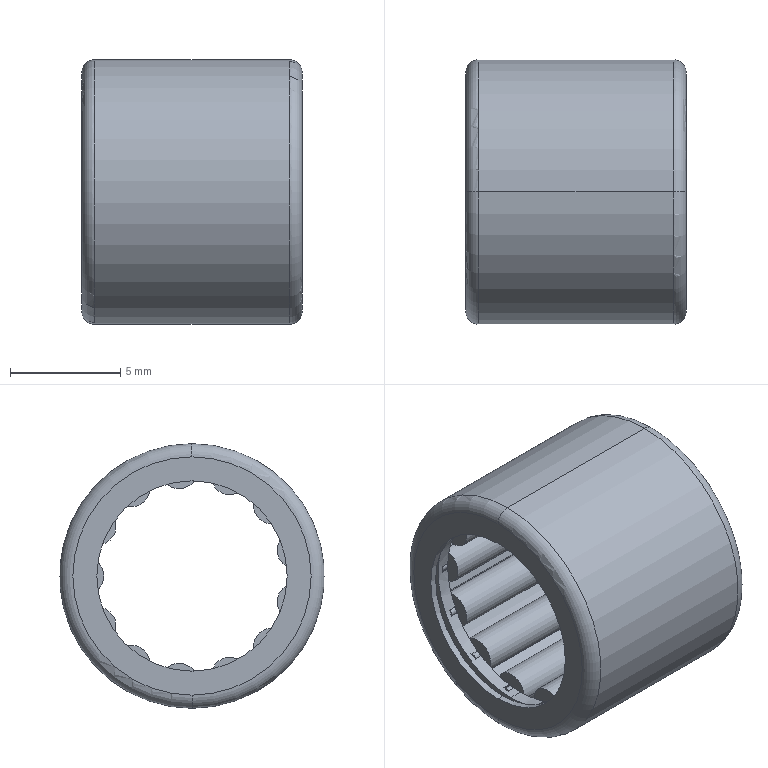Part | SolidWorks | features Revolution 3, CirPattern 2, MirrorPattern 2, Fillet 1, RevCut 1 | 1 solid | 221 faces | box 10 x 12 x 12 mm | volume 357.664 mm3 | cylinder 120 | plane 97 | torus 4 | commonest cylinder face diameters 0.475 x39 1.69 x27 0.375 x26 1.689 x12 8.625 x4 9.312 x4